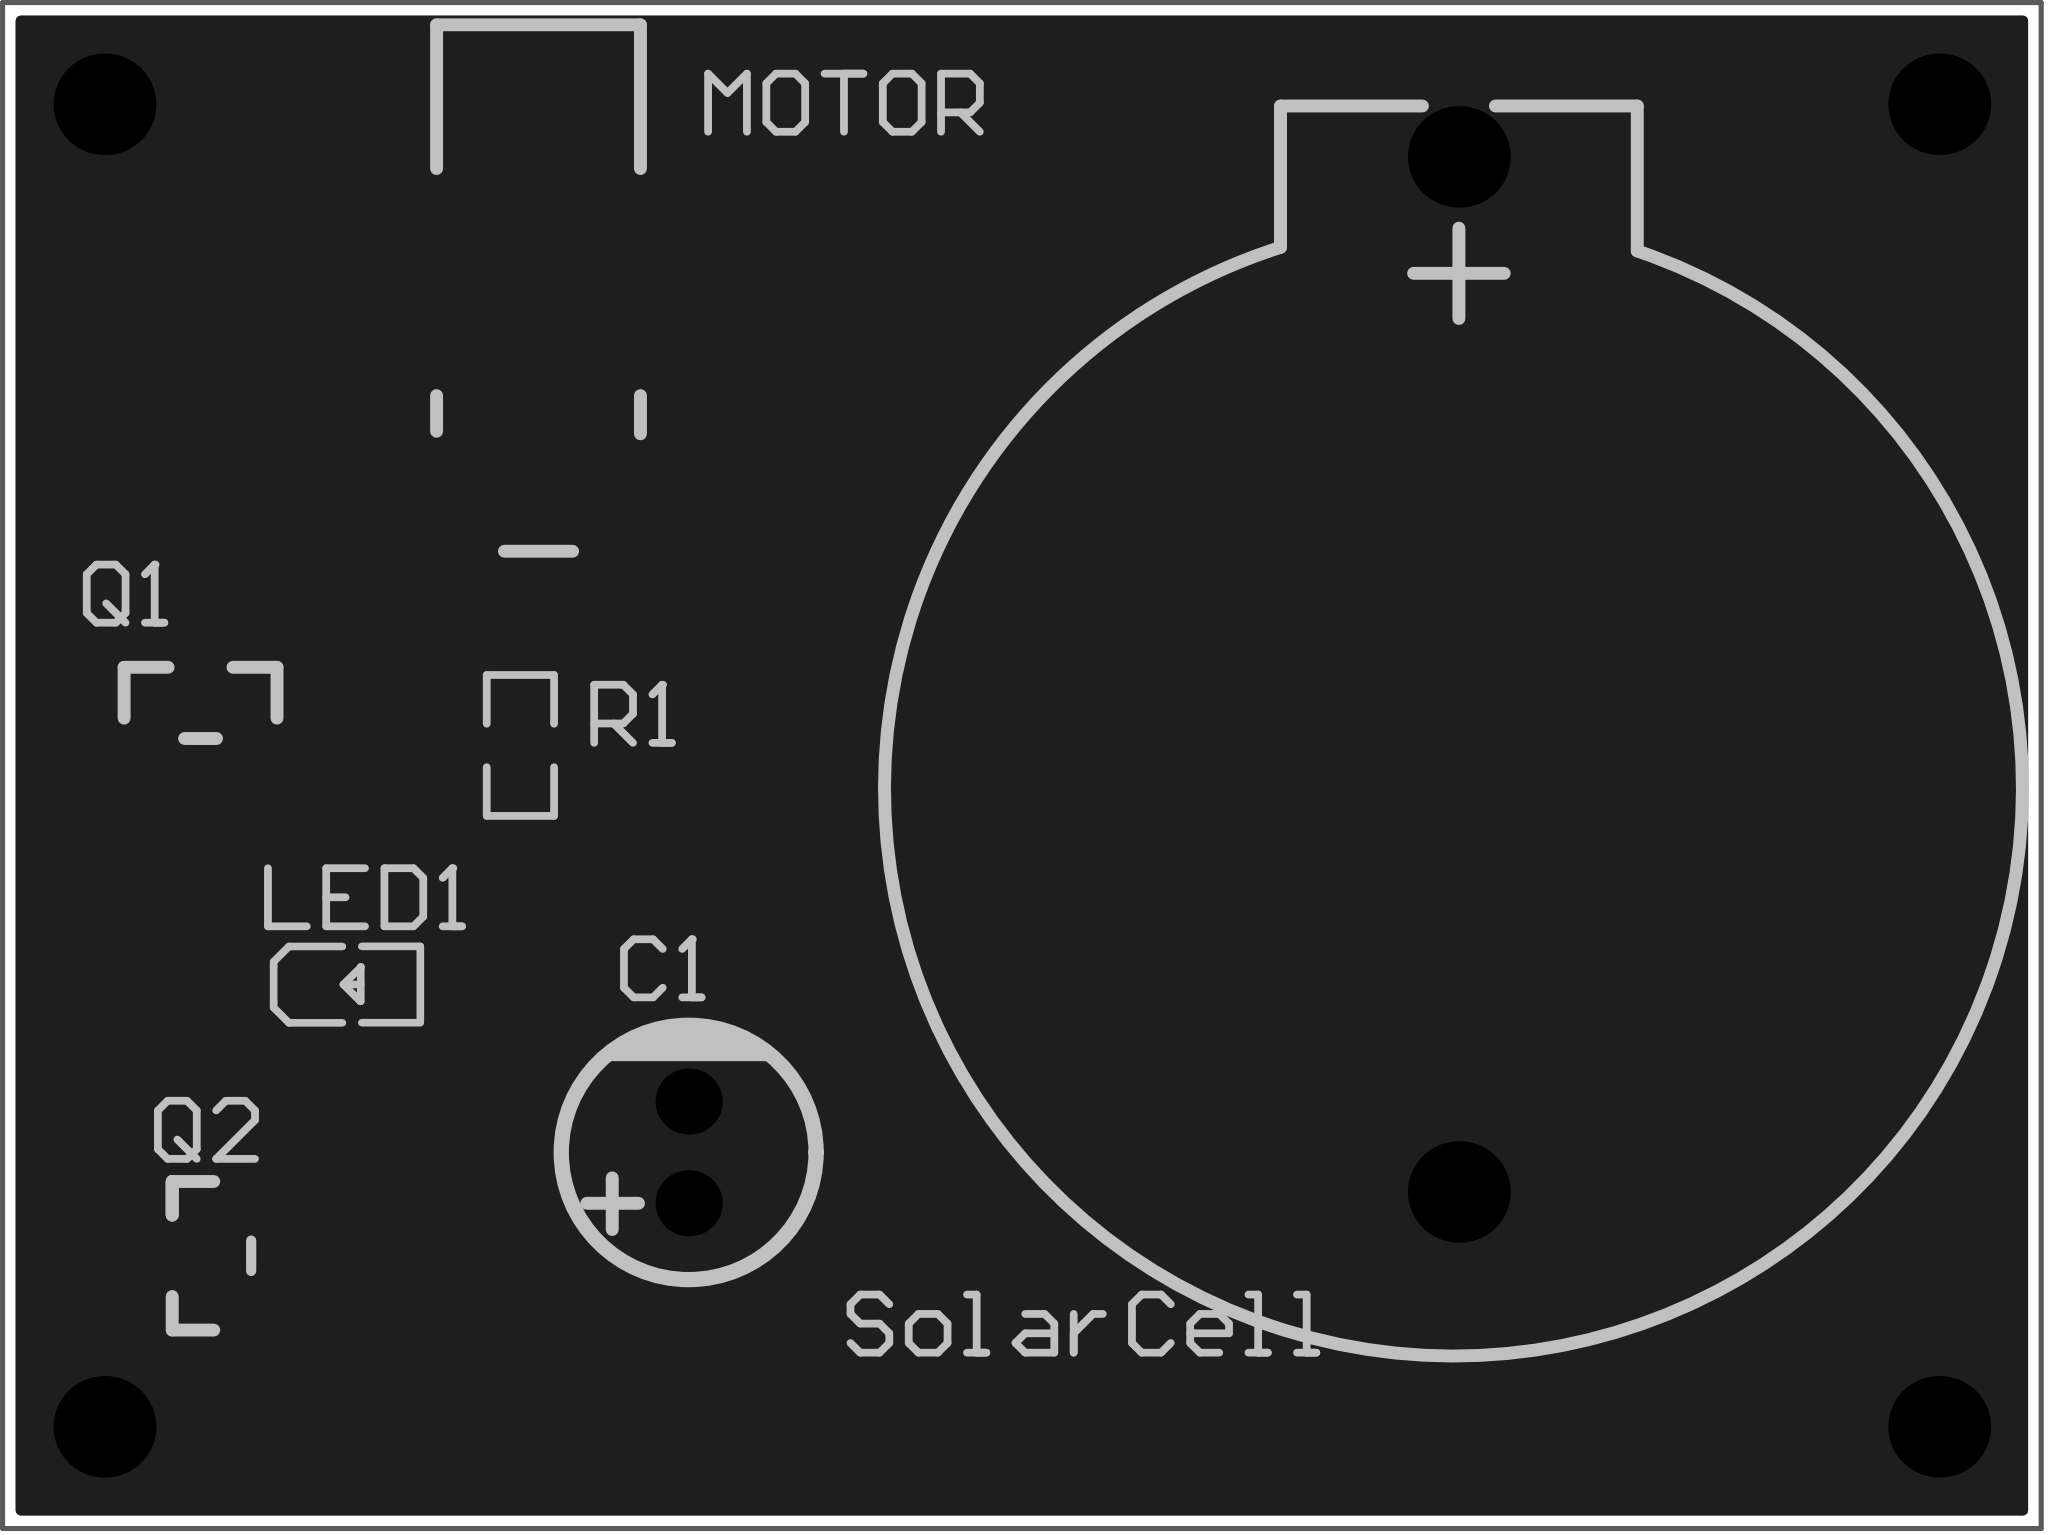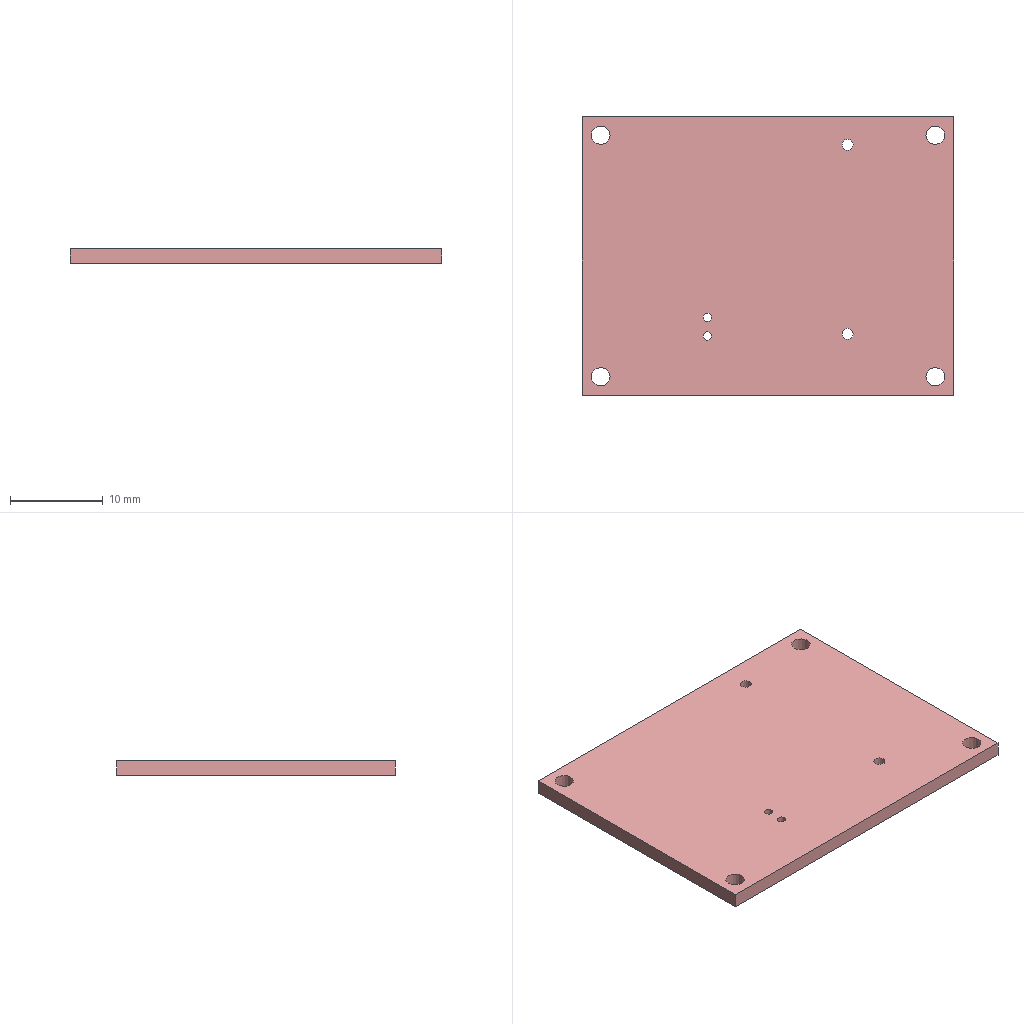Circuit board layout | Altium Designer | box 40 x 30 x 1.6 mm
Layer stack:
# Altium Designer layer stack of  (unit mm; dielectric type: 0 none, 1 core, 2 prepreg, 3 surface material)
index,name,kind,layer,copper_thickness_mm,dielectric_type,dielectric_thickness_mm,dielectric_material,dielectric_constant
0,Top Paste Mask Layer,other,,,,,,
1,Top Silkscreen Layer,other,,,,,,
2,Top Solder Mask Layer,dielectric,,,3,0.01,,3.3
3,Top Layer,copper,Top Layer,0.035,,,,
4,Dielectric1,dielectric,,,3,1.51,FR4,4.5
5,Bottom Layer,copper,Bottom Layer,0.035,,,,
6,Bottom Solder Mask Layer,dielectric,,,3,0.01,,3.3
7,Bottom Silkscreen Layer,other,,,,,,
8,Bottom Paste Mask Layer,other,,,,,,
# drill layer pairs: low layer,high layer
drill_pair,Top Layer,Bottom Layer
Part placement:
Designator,Comment,Layer,Footprint,Center-X(mm),Center-Y(mm),Rotation
C1,4700uF,TopLayer,CAP-TH_BD5.0-P2.00-D0.8-FD-10UF50VC110GL,93.345,87.122,90
LED1,,TopLayer,LED_0603,86.69,90.416,0
MOTOR,MOTOR_3,TopLayer,VIBRATING-MOTOR-SMD_3P_C9900012555,90.399,102.15,270
Q1,,TopLayer,S8050_SOT-23,83.767,95.959,270
Q2,,TopLayer,S8550P_SOT,83.862,85.09,0
R1,2.2K,TopLayer,R0603,90.043,95.123,90
SolarCell,1.5V*2,TopLayer,BAT-TH_CR2032-2-1,108.458,96.52,90
Pad and via stacks:
# Altium Designer via and pad stacks of  (unit mm). Each distinct definition once, with the count of objects using it.
# via: kind,start_layer,end_layer,hole_mm,diameter_mm,mode(0 simple;1 top-mid-bottom;2 full stack),diameter_per_layer,count,example_net
# pad: kind,layer,hole_mm,hole_type(0 round;1 square;2 slot),plating,top_size,top_shape(1 round;2 rect;3 octagon;9 rounded rect),mid_size,bottom_size,mode,footprint,size_per_layer,count,example
pad,Multi-Layer,0.9,0,plated,1.3x1.3,1,1.3x1.3,1.3x1.3,0,CAP-TH_BD5.0-P2.00-D0.8-FD-10UF50VC110GL,,2,C1.2
pad,Multi-Layer,1.2,0,plated,2x2,1,2x2,2x2,0,BAT-TH_CR2032-2-1,,2,SolarCell.2
pad,Multi-Layer,2,0,plated,2x2,1,2x2,2x2,0,,,4,1
pad,Top Layer,0,0,plated,0.8001x0.8001,2,0.8001x0.8001,0.8001x0.8001,0,LED_0603,,2,LED1.1
pad,Top Layer,0,0,plated,4x4.5,2,4x4.5,4x4.5,0,VIBRATING-MOTOR-SMD_3P_C9900012555,,1,MOTOR.3
pad,Top Layer,0,0,plated,2x1.5,2,2x1.5,2x1.5,0,VIBRATING-MOTOR-SMD_3P_C9900012555,,2,MOTOR.2
pad,Top Layer,0,0,plated,1x0.8,2,1x0.8,1x0.8,0,S8050_SOT-23,,3,Q1.2
pad,Top Layer,0,0,plated,0.701x1.25,2,0.701x1.25,0.701x1.25,0,S8550P_SOT,,3,Q2.3
pad,Top Layer,0,0,plated,0.8065x0.864,2,0.8065x0.864,0.8065x0.864,0,R0603,,2,R1.2
Copper pours:
name,layer,net,type(0 solid;1 hatched;2 none)
Top Layer-$1N1,Top Layer,$1N1,0
Bottom Layer-$1N1,Bottom Layer,$1N1,0
Design rules, without the lines most boards share:
# Altium Designer design rules of  (exported by Altium Designer, unit mm)
# columns: name | kind | enabled | priority | scope1 | scope2 | descriptor | typed fields (field=value)
creepage | 65 | enabled | 1 | All | All | Creepage Distance Constraint =(0mil) (All),(All) |
copperRegion | 20 | enabled | 1 | (InNet('$1N1')) | All | Polygon Connect Rule(Relief Connect )(Conductor Width=10mil) (Relief Angle=90 Angle) (Entries=4) (Air Gap Width=10mil) ((InNet('$1N1'))),(All) | connect_style(0=relief,1=direct,2=none)=0 relief_conductor_width=0.254 relief_entries=4